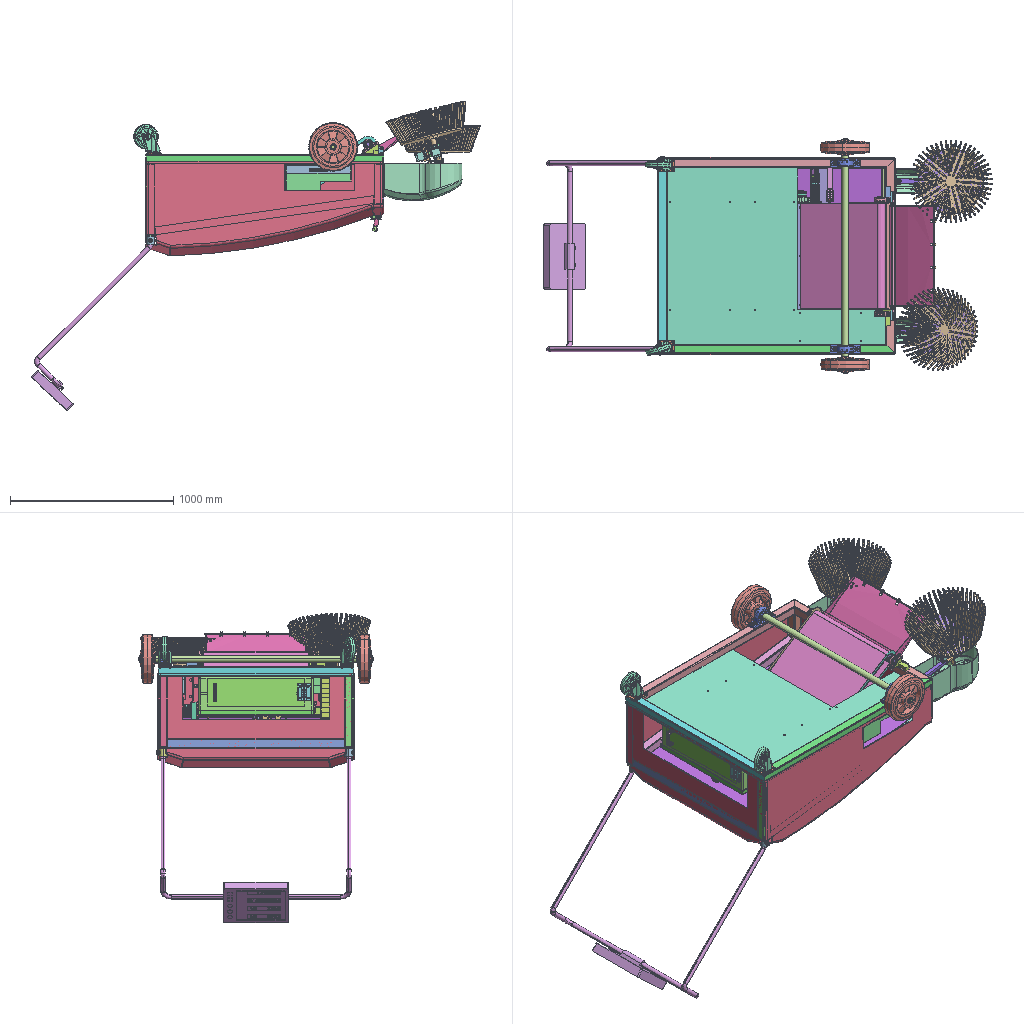Assembly | SolidWorks | 107 different items | 175 placed | box 2749 x 1446 x 1897 mm
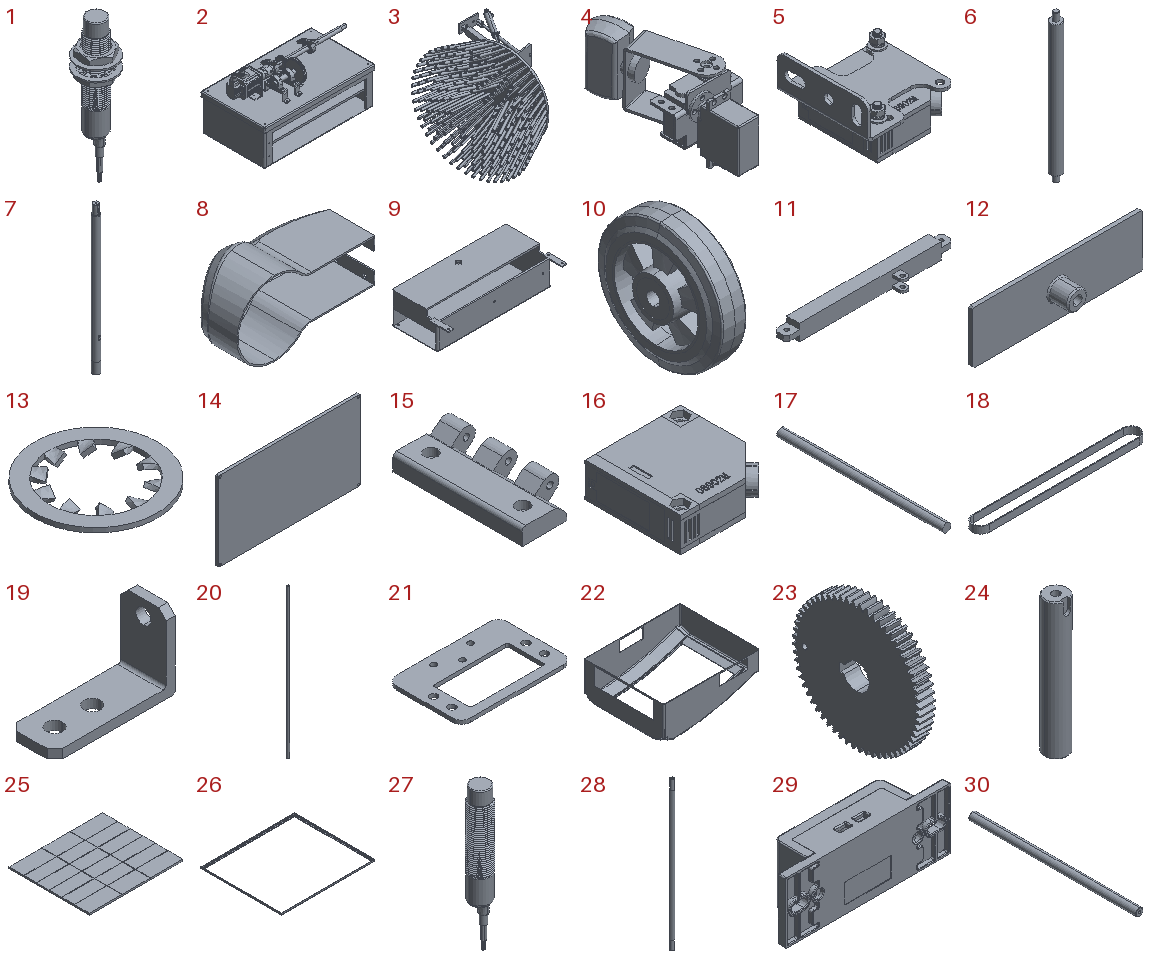Parts list (item | name | quantity | parent item | size | volume | features):
1 | (subassembly) | x1 | - | 21.5 x 21.5 x 81 mm | 7129 mm3 | features CompositeCurve 7
2 | (subassembly) | x1 | - | 752 x 410 x 396 mm | 13592742 mm3 | features CompositeCurve 2
3 | (subassembly) | x1 | - | 492.003 x 639.962 x 507.373 mm | 6091751 mm3 | -
4 | (subassembly) | x1 | - | 62.179 x 144.352 x 61.763 mm | 114357 mm3 | features MirrorCompFeat 1
5 | (subassembly) | x1 | - | 60 x 58 x 40 mm | 49039 mm3 | features CompositeCurve 4
6 | - | x1 | - | 55 x 55 x 730 mm | 1583008 mm3 | features Chamfer 1, Extrusion 1, ICE 1, MirrorPattern 1
7 | - | x1 | - | 25 x 25 x 522 mm | 247598 mm3 | features ICE 4, Chamfer 1, Extrusion 1, Fillet 1, HoleWzd 1
8 | - | x2 | - | 480 x 231.625 x 260 mm | 1531770 mm3 | features Fillet 2, ICE 2, Chamfer 1, Extrusion 1, Shell 1
9 | - | x1 | - | 730 x 359.087 x 200 mm | 6377520 mm3 | features ICE 5, HoleWzd 3, Extrusion 1, Fillet 1, Shell 1
10 | - | x2 | - | 90 x 300 x 300 mm | 3470694 mm3 | features BaseBody 1, Scale 1
11 | - | x2 | - | 260 x 36.5 x 25 mm | 116892 mm3 | features ICE 3, Chamfer 1, Extrusion 1, LPattern 1, MirrorPattern 1
12 | - | x1 | - | 130 x 18 x 40 mm | 17593 mm3 | features Chamfer 1, Extrusion 1, HoleWzd 1, ICE 1
13 | - | x2 | in 1 | 21.5 x 21.5 x 1.797 mm | 153.883 mm3 | features CirPattern 1, Extrusion 1, Helix 1, Sweep 1
14 | - | x1 | - | 680 x 47 x 380 mm | 3131077 mm3 | features ICE 5, Chamfer 1, Extrusion 1
15 | - | x2 | - | 47.1 x 102 x 20.1 mm | 51608 mm3 | features MBimport 1
16 | - | x1 | in 5 | 50 x 50 x 18 mm | 41624 mm3 | features ICE 29, LPattern 4, CirPattern 2, Fillet 2, Chamfer 1, Extrusion 1, MirrorPattern 1
17 | - | x1 | - | 5 x 99 x 5 mm | 1944 mm3 | features MBimport 1
18 | - | x1 | - | 667 x 67 x 27 mm | 113486 mm3 | features Extrusion 1
19 | - | x2 | - | 80 x 30 x 50 mm | 20408 mm3 | features Chamfer 1, Extrusion 1, Fillet 1, ICE 1
20 | - | x1 | - | 10 x 10 x 700 mm | 54949 mm3 | features Chamfer 1, Extrusion 1
21 | - | x1 | - | 60 x 40 x 2 mm | 2957 mm3 | features ICE 3, Extrusion 1
22 | - | x1 | - | 1460 x 1210 x 578.799 mm | 14635130 mm3 | features ICE 7, Chamfer 3, Fillet 2, MoveFace 2, Shell 1
23 | - | x1 | - | 15 x 123.892 x 123.892 mm | 159845 mm3 | features HoleWzd 1, MBimport 1
24 | - | x1 | - | 25 x 25 x 150 mm | 71725 mm3 | features Chamfer 1, Extrusion 1, Fillet 1, HoleWzd 1, ICE 1
25 | - | x1 | - | 1340 x 1150 x 55 mm | 38292286 mm3 | features ICE 3, Extrusion 1, LPattern 1, Sweep 1
26 | - | x1 | - | 1348 x 1158 x 25 mm | 890268 mm3 | features WeldMemberFeat 1, WeldmentFeature 1
27 | - | x1 | in 1 | 11.9 x 11.9 x 81 mm | 5802 mm3 | features Fillet 4, ICE 4, Revolution 4, Helix 1, SweepCut 1
28 | - | x1 | - | 40 x 40 x 1420 mm | 1677021 mm3 | features HoleWzd 2, Chamfer 1, Extrusion 1, ICE 1
29 | - | x1 | - | 40.625 x 10.25 x 15 mm | 2277 mm3 | features BaseBody 3, CombineBodies 1, MoveFace 1, Scale 1
30 | - | x4 | - | 10 x 220 x 10 mm | 17093 mm3 | features HoleWzd 2, Chamfer 1, Extrusion 1
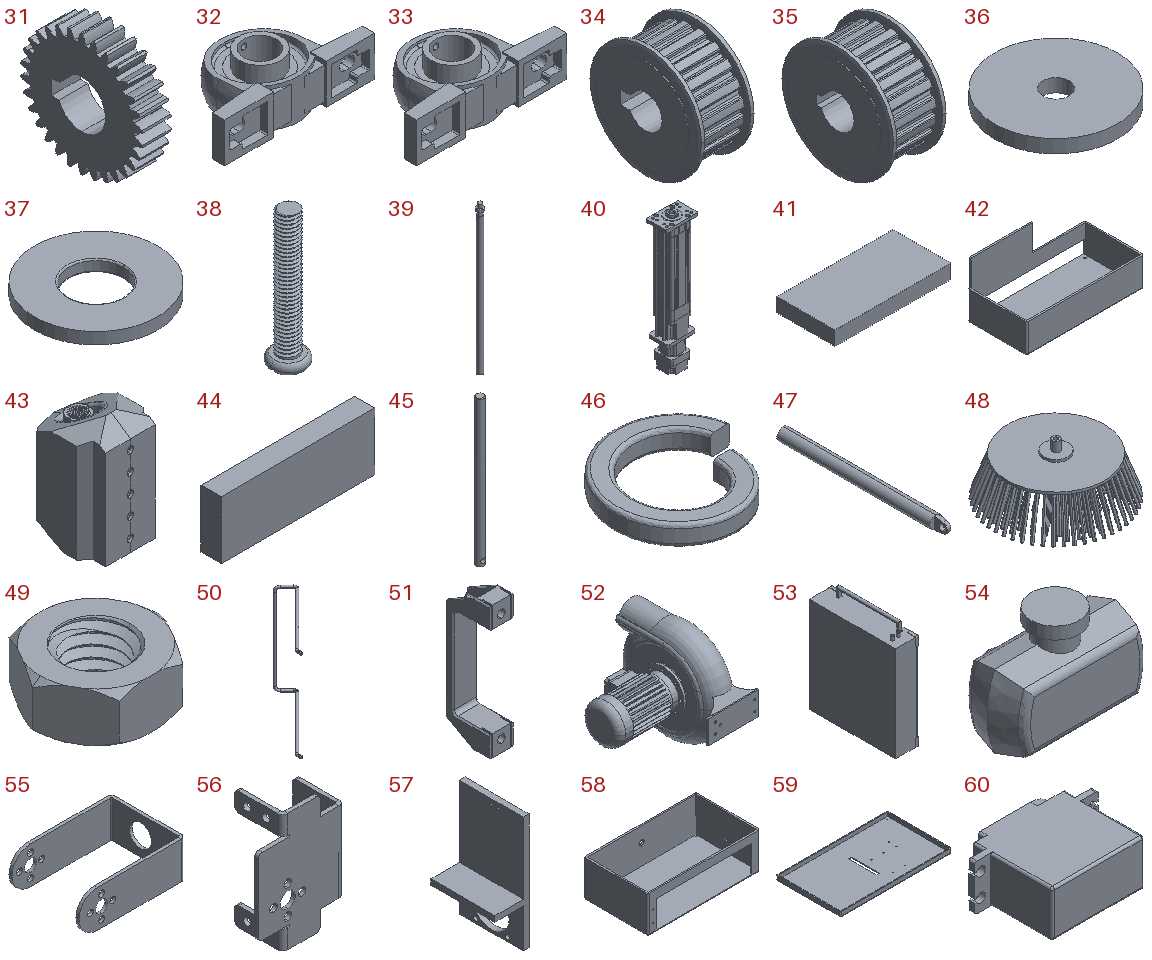31 | - | x1 | - | 15 x 63.764 x 64 mm | 33715 mm3 | features MBimport 1
32 | - | x2 | - | 186 x 100.8 x 54.842 mm | 267001 mm3 | features Revolution 5, Boss 3, Cut 3, RevCut 2, CirPattern 1, Extrusion 1, SweepCut 1
33 | - | x8 | - | 116.25 x 63 x 34.276 mm | 65186 mm3 | features Revolution 5, Boss 3, Cut 3, RevCut 2, CirPattern 1, Extrusion 1, Scale 1, SweepCut 1
34 | - | x1 | - | 32 x 67 x 67 mm | 76462 mm3 | features ICE 1, MBimport 1
35 | - | x2 | - | 32 x 67 x 67 mm | 77303 mm3 | features ICE 1, MBimport 1
36 | - | x2 | - | 28 x 28 x 3 mm | 1762 mm3 | features Extrusion 1
37 | - | x2 | in 5 | 9.05 x 9.05 x 0.85 mm | 43.941 mm3 | features Extrusion 1, Fillet 1, ICE 1
38 | - | x2 | in 5 | 6.8 x 6.8 x 27.2 mm | 311.216 mm3 | features ICE 4, Chamfer 1, Extrusion 1, Fillet 1, Helix 1, RevCut 1, Revolution 1, SweepCut 1
39 | - | x1 | - | 12 x 13.856 x 280 mm | 21775 mm3 | features MBimport 1, MoveFace 1, Scale 1
40 | - | x1 | - | 66 x 42 x 279.6 mm | 278895 mm3 | features MBimport 1, MoveFace 1
41 | - | x1 | - | 390 x 195 x 47.5 mm | 741654 mm3 | features Extrusion 1, Shell 1
42 | - | x1 | - | 400 x 200 x 190 mm | 953105 mm3 | features ICE 3, Fillet 2, Extrusion 1, Shell 1
43 | - | x1 | - | 45.232 x 51.14 x 74.295 mm | 38659 mm3 | features BaseBody 6
44 | - | x1 | - | 690 x 90 x 260 mm | 2021904 mm3 | features Extrusion 1, Shell 1
45 | - | x2 | - | 8 x 8 x 150 mm | 7385 mm3 | features Chamfer 1, Extrusion 1, ICE 1
46 | - | x2 | in 5 | 6.6 x 6.6 x 2.189 mm | 20.119 mm3 | features Helix 1, Sweep 1
47 | - | x2 | - | 12 x 163 x 12 mm | 9872 mm3 | features ICE 2, Extrusion 1, Shell 1
48 | - | x2 | - | - | - | features CirPattern 7, ICE 3, CombineBodies 1, Extrusion 1, Fillet 1, LPattern 1, OffsetRefSurface 1, ReplaceFace 1, Sweep 1
49 | - | x2 | in 5 | 7.91 x 6.85 x 3.05 mm | 87.239 mm3 | features Chamfer 1, Extrusion 1, Helix 1, ICE 1, RevCut 1, SweepCut 1
50 | - | x1 | - | 724.68 x 923.528 x 1170 mm | 1404787 mm3 | features 3DProfileFeature 3, Cut 1, Shell 1, Sweep 1
51 | - | x3 | - | 20 x 36 x 110 mm | 17645 mm3 | features MBimport 1
52 | - | x1 | - | - | - | features DeleteBody 6, MoveCopyBody 4, MBimport 1, Scale 1
53 | - | x1 | - | 36 x 137.7 x 182.4 mm | 710177 mm3 | features ICE 1, MBimport 1, Scale 1
54 | - | x1 | in 4 | - | - | features ICE 4, Fillet 3, Extrusion 1, RevolvRefSurf 1
55 | - | x1 | in 4 | 71.712 x 49.895 x 25 mm | 8226 mm3 | features ICE 3, FlatPattern 1, SM3dBend 1, SMBaseFlange 1, SheetMetal 1
56 | - | x1 | in 4 | 45 x 25 x 62 mm | 6846 mm3 | features ICE 5, Fillet 3, EdgeFlange 2, SMBaseFlange 2, FlatPattern 1, MirrorPattern 1, SheetMetal 1
57 | - | x2 | - | 48 x 90 x 163 mm | 129456 mm3 | features ICE 3, Cut 2, Extrusion 1, HoleWzd 1
58 | - | x1 | - | 700 x 400 x 230 mm | 6454208 mm3 | features Cut 4, HoleWzd 3, Extrusion 1, Fillet 1, Shell 1
59 | - | x1 | - | 710 x 410 x 30 mm | 1701440 mm3 | features Cut 1, Extrusion 1, Fillet 1, HoleWzd 1, ICE 1, Shell 1
60 | - | x2 | in 4 | 54 x 43 x 20 mm | 30390 mm3 | features ICE 5, 3DProfileFeature 1, Extrusion 1, Fillet 1, HoleWzd 1
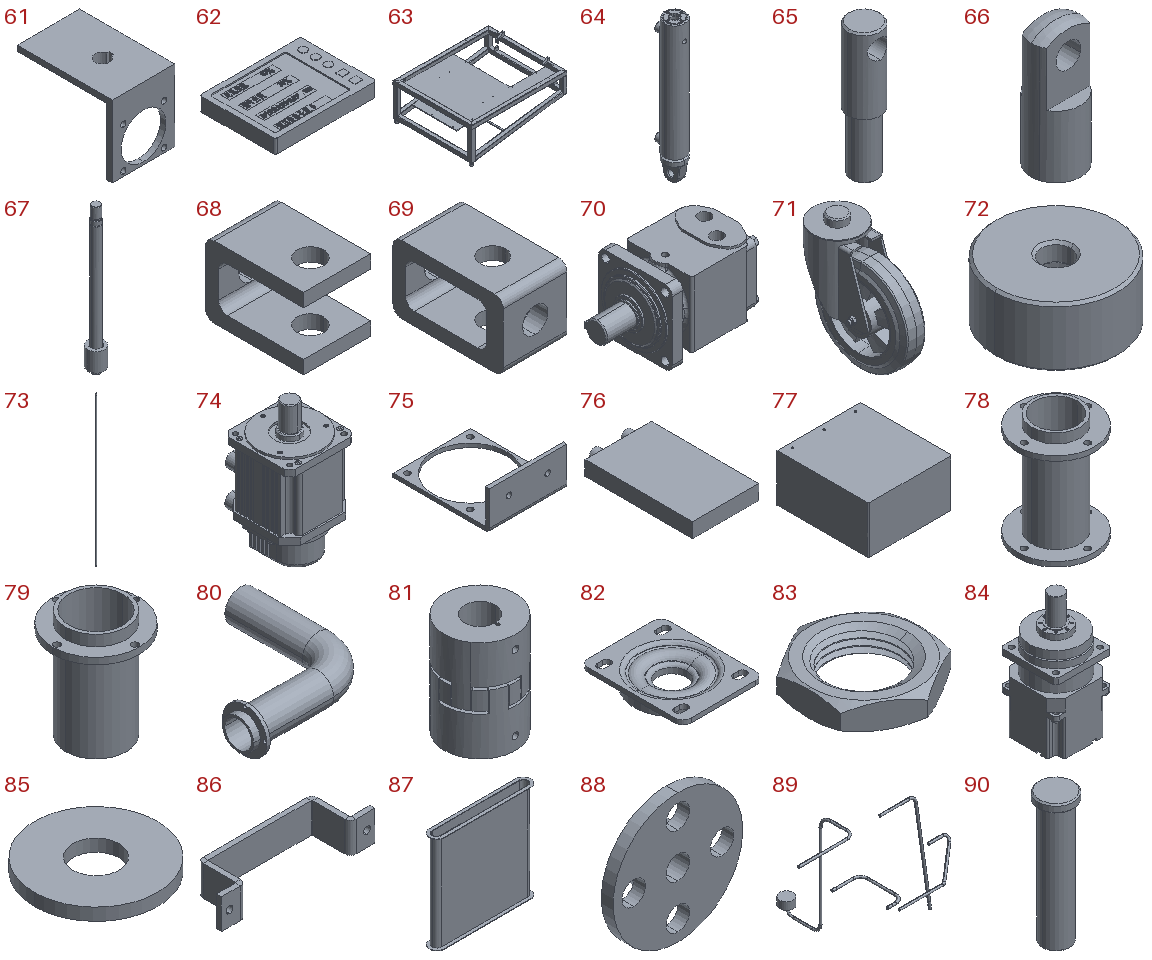61 | - | x2 | - | 70 x 106 x 80 mm | 69922 mm3 | features ICE 3, Cut 1, Extrusion 1
62 | - | x1 | - | 400 x 300 x 104.5 mm | 6453312 mm3 | features ICE 7, Extrusion 1, Fillet 1, HoleWzd 1
63 | - | x1 | - | 1460 x 1200 x 621.009 mm | 23985037 mm3 | features ICE 14, MoveCopyBody 6, WeldMemberFeat 4, Fillet 3, HoleWzd 3, BossThin 2, Cut 2, EndCap 2, MirrorSolid 2, WeldCornerFeat 2, WeldmentFeature 1
64 | - | x2 | - | 22 x 28 x 150.8 mm | 29606 mm3 | features BaseBody 4, CombineBodies 1, Scale 1
65 | - | x1 | - | 10 x 10 x 41 mm | 2435 mm3 | features ICE 2, Chamfer 1, Extrusion 1
66 | - | x2 | - | 12 x 12 x 30 mm | 1906 mm3 | features MBimport 1, MoveFace 1, Scale 1
67 | - | x2 | - | 15.92 x 15.92 x 140.8 mm | 10674 mm3 | features BaseBody 2, CombineBodies 1, Scale 1
68 | - | x1 | - | 15 x 22 x 16 mm | 2176 mm3 | features ICE 2, Extrusion 1, Fillet 1
69 | - | x1 | - | 15 x 26 x 16 mm | 3022 mm3 | features ICE 3, Fillet 2, Extrusion 1
70 | - | x4 | - | 102 x 56 x 56 mm | 177748 mm3 | features ICE 1, MBimport 1, Scale 1
71 | - | x2 | - | 77.25 x 166.125 x 185.063 mm | 534809 mm3 | features BaseBody 4, CombineBodies 2, ICE 2, Chamfer 1, MoveCopyBody 1, MoveFace 1, Scale 1
72 | - | x4 | - | 25 x 25 x 12 mm | 4138 mm3 | features Chamfer 1, Cut 1, Extrusion 1
73 | - | x1 | - | 5 x 5 x 632 mm | 12318 mm3 | features Chamfer 1, Extrusion 1, ICE 1, MirrorPattern 1
74 | - | x1 | - | 100 x 136 x 194 mm | 1174921 mm3 | features ICE 1, MBimport 1
75 | - | x1 | - | 100 x 125 x 50 mm | 47710 mm3 | features Cut 1, EdgeFlange 1, FlatPattern 1, ICE 1, SMBaseFlange 1, SheetMetal 1
76 | - | x8 | - | 135 x 235 x 30 mm | 903464 mm3 | features Extrusion 1, ICE 1
77 | - | x1 | - | 252 x 276 x 143 mm | 499174 mm3 | features SMBaseFlange 3, SheetMetal 3, CombineBodies 1, Cut 1, Fillet 1, FlatPattern 1, HoleWzd 1
78 | - | x1 | - | 80 x 80 x 120 mm | 82655 mm3 | features Extrusion 1, ICE 1, MirrorPattern 1
79 | - | x1 | - | 40 x 40 x 50 mm | 8082 mm3 | features Extrusion 1, ICE 1
80 | - | x1 | - | 116 x 120 x 40 mm | 32734 mm3 | features ICE 1, Shell 1, Sweep 1
81 | - | x1 | - | 55 x 55 x 78 mm | 139645 mm3 | features ICE 1, MBimport 1
82 | - | x2 | - | 82.5 x 105 x 14.438 mm | 61756 mm3 | features BaseBody 4, CombineBodies 2, ICE 2, MoveCopyBody 1, MoveFace 1, Scale 1
83 | - | x2 | in 1 | 16.5 x 19.053 x 4 mm | 509.412 mm3 | features Helix 1, ICE 1, RevCut 1, Revolution 1, SweepCut 1
84 | - | x1 | - | 30 x 37.375 x 65.875 mm | 38357 mm3 | features BaseBody 3, CombineBodies 1, Scale 1
85 | - | x2 | - | 40 x 40 x 4 mm | 4320 mm3 | features Extrusion 1
86 | - | x2 | - | 156.25 x 44.25 x 30.75 mm | 34854 mm3 | features FlatPattern 1, ICE 1, SMBaseFlange 1, SheetMetal 1
87 | - | x1 | - | 680 x 100 x 650 mm | 2347902 mm3 | features Extrusion 1, ICE 1, MirrorSolid 1
88 | - | x2 | in 4 | 22 x 6 x 22 mm | 838.805 mm3 | features ICE 2, Extrusion 1
89 | - | x1 | - | 155.715 x 218.5 x 171.95 mm | 7637 mm3 | features 3DProfileFeature 5, Sweep 4, ICE 1
90 | - | x1 | - | 13 x 13 x 48 mm | 3919 mm3 | features Chamfer 1, Extrusion 1, ICE 1
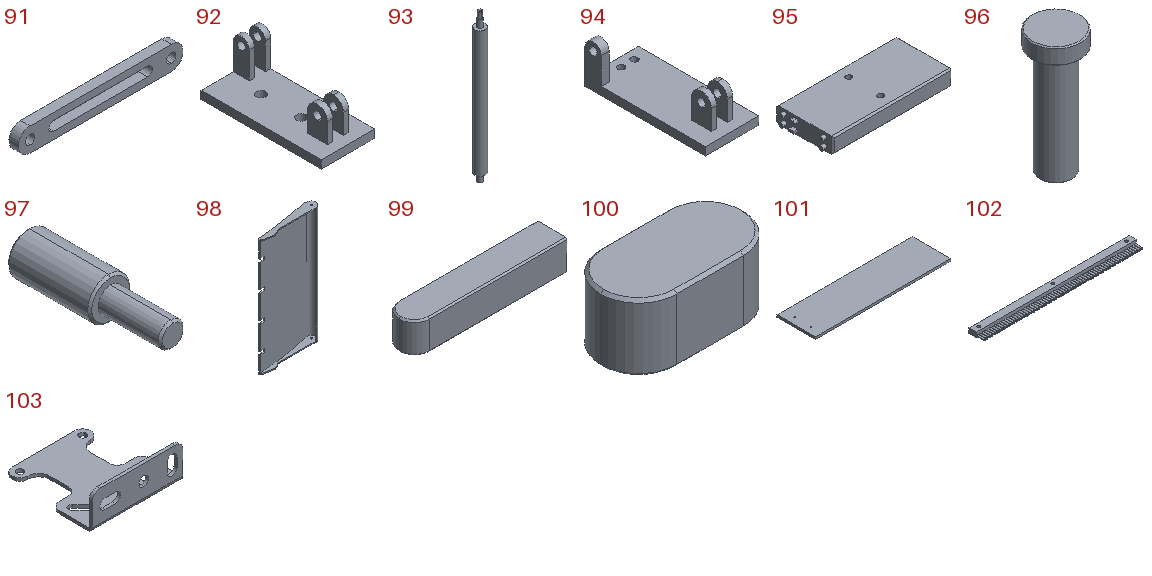91 | - | x1 | - | 175 x 10 x 25 mm | 30053 mm3 | features Extrusion 1, ICE 1
92 | - | x2 | - | 40 x 90 x 32 mm | 25565 mm3 | features ICE 3, Extrusion 1, LPattern 1, MirrorPattern 1
93 | - | x1 | - | 55 x 55 x 762 mm | 1592560 mm3 | features ICE 3, Chamfer 2, Extrusion 1, HoleWzd 1, MirrorPattern 1
94 | - | x2 | - | 40 x 90 x 32 mm | 25255 mm3 | features ICE 3, Extrusion 1, MirrorPattern 1
95 | - | x1 | - | 155 x 70 x 20 mm | 207430 mm3 | features ICE 2, Chamfer 1, Extrusion 1
96 | - | x12 | - | 9 x 9 x 23 mm | 754.856 mm3 | features Chamfer 1, Extrusion 1, ICE 1
97 | - | x1 | - | 10 x 35 x 10 mm | 1985 mm3 | features Chamfer 1, Extrusion 1, ICE 1
98 | - | x1 | - | 325.159 x 69.885 x 620 mm | 1237275 mm3 | features Fillet 3, ICE 3, Extrusion 1, MirrorPattern 1, Shell 1
99 | - | x2 | - | 30 x 6 x 6 mm | 1051 mm3 | features Chamfer 1, Extrusion 1, Fillet 1
100 | - | x2 | - | 15 x 8 x 7 mm | 740.393 mm3 | features Chamfer 1, Extrusion 1, Fillet 1
101 | - | x1 | - | 600 x 170 x 10 mm | 1019607 mm3 | features Extrusion 1, HoleWzd 1
102 | - | x1 | - | 650 x 60 x 20 mm | 429985 mm3 | features ICE 3, Fillet 2, Extrusion 1, LPattern 1, Sweep 1
103 | - | x1 | in 5 | 58 x 60 x 22 mm | 6510 mm3 | features ICE 3, MirrorPattern 2, SketchHole 2, EdgeFlange 1, Fillet 1, FlatPattern 1, SMBaseFlange 1, SheetMetal 1
104 | deep groove ball bearings gb | x1 | - | - | - | -
105 | hex nuts, style 1-grades ab gb | x1 | - | - | - | -
106 | hexagon head bolts-full thread gb | x1 | - | - | - | -
107 | hexagon socket head cap screws gb | x1 | - | - | - | -
Mates (type | each side: item.copy, entity, surface, feature):
In the top assembly
Coincident | 63.1 plane | assembly plane | 6 times
Width | 25.1 face plane Boss-Extrude1 | 25.1 face plane Boss-Extrude1 | 63.1 face plane Square tube - configured 80 X 80 X 5(4) | 63.1 face plane Body-Move/Copy5
Width | 9.1 face plane Boss-Extrude1 | 9.1 face plane Boss-Extrude1 | 63.1 face plane Square tube - configured 80 X 80 X 5(1) | 63.1 face plane Square tube - configured 80 X 80 X 5(1)
Concentric | 10.1 face cylinder RE.G2-200-RSL.step-1/RE-G2-L.step-1-solid1 | 10.2 face cylinder RE.G2-200-RSL.step-1/RE-G2-L.step-1-solid1
DistanceDim | 10.1 face plane RE.G2-200-RSL.step-1/RE-G2-L.step-1-solid1 | 63.1 face plane Square tube - configured 80 X 80 X 5(1)
DistanceDim | 10.2 face plane RE.G2-200-RSL.step-1/RE-G2-L.step-1-solid1 | 63.1 face plane Square tube - configured 80 X 80 X 5(1)
Concentric | 10.1 face cylinder RE.G2-200-RSL.step-1/RE-G2-L.step-1-solid1 | 28.1 face cylinder Boss-Extrude3
Width | 28.1 face plane Boss-Extrude1 | 28.1 face plane Boss-Extrude1 | 10.2 face plane RE.G2-200-RSL.step-1/RE-G2-L.step-1-solid1 | 10.1 face plane RE.G2-200-RSL.step-1/RE-G2-L.step-1-solid1
Concentric | 32.1 face cylinder Boss-Revolve5 | 28.1 face cylinder Boss-Extrude3
Concentric | 28.1 face cylinder Boss-Extrude3 | 32.2 face cylinder Boss-Revolve5
Coincident | 32.1 face plane Boss-Extrude1 | 32.2 face plane Boss-Extrude1
Coincident | 63.1 face plane Square tube - configured 80 X 80 X 5(1) | 32.1 face plane Boss-Extrude1
Width | 32.1 face plane Boss-Extrude1 | 32.1 face plane Boss-Extrude1 | 63.1 face plane Square tube - configured 80 X 80 X 5(1) | 63.1 face plane Square tube - configured 80 X 80 X 5(1)
Width | 32.2 face plane Boss-Extrude1 | 32.2 face plane Boss-Extrude1 | 63.1 face plane Square tube - configured 80 X 80 X 5(1) | 63.1 face plane Square tube - configured 80 X 80 X 5(1)
Width | 87.1 face plane Boss-Extrude1 | 87.1 face plane Boss-Extrude1 | 63.1 face plane Square tube - configured 80 X 80 X 5(4) | 63.1 face plane Body-Move/Copy5
Concentric | 87.1 face cylinder Boss-Extrude1 | 6.1 face cylinder Boss-Extrude1
Coincident | 87.1 face plane Boss-Extrude1 | 6.1 face plane Boss-Extrude1
Concentric | 87.1 face cylinder Boss-Extrude1 | 93.1 face cylinder Boss-Extrude1
Coincident | 87.1 face plane Boss-Extrude1 | 93.1 face plane Boss-Extrude1
Concentric | 6.1 face cylinder Boss-Extrude2 | 33.1 face cylinder Boss-Revolve5
Concentric | 6.1 face cylinder Mirror1 | 33.2 face cylinder Boss-Revolve5
Coincident | 33.2 face plane Boss-Extrude1 | 33.1 face plane Boss-Extrude1
Coincident | 6.1 face plane Boss-Extrude2 | 33.1 face plane Boss-Revolve5
Coincident | 6.1 face plane Mirror1 | 33.2 face plane Boss-Revolve5
Concentric | 93.1 face cylinder Boss-Extrude2 | 33.3 face cylinder Boss-Revolve5
Concentric | 93.1 face cylinder Mirror1 | 33.4 face cylinder Boss-Revolve5
Coincident | 33.3 face plane Boss-Extrude1 | 33.4 face plane Boss-Extrude1
Coincident | 93.1 face plane Boss-Extrude2 | 33.3 face plane Boss-Revolve5
Coincident | 93.1 face plane Mirror1 | 33.4 face plane Boss-Revolve5
Parallel | 63.1 face plane Square tube - configured 80 X 80 X 5(1) | 33.3 face plane Boss-Extrude1
Coincident | 76.1 face plane Boss-Extrude1 | 77.1 face plane Base-Flange1 | 2 times
Coincident | 76.1 face plane Boss-Extrude1 | 77.1 face plane Base-Flange3
Concentric | 63.1 face cylinder Boss-Extrude1 | 50.1 face cylinder Sweep1 | 2 times
Coincident | 63.1 face plane Square tube - configured 80 X 80 X 5(3) | 50.1 face plane Sweep1
Coincident | 71.1 face plane Cut-Extrude1 | 82.1 face plane Caster with Brake.STEP-1/RE.G2-200-SSF-H.step.STEP-1/RE-G2-SSF-H-ZL.step.STEP-1-solid1
Concentric | 71.1 face cylinder Caster with Brake.STEP-1/RE.G2-200-SSF-H.step.STEP-1/RE-G2-SSF-H-ZL.step.STEP-1-solid1 | 82.1 face cylinder Caster with Brake.STEP-1/RE.G2-200-SSF-H.step.STEP-1/RE-G2-SSF-H-ZL.step.STEP-1-solid1
Coincident | 63.1 face plane Square tube - configured 80 X 80 X 5(1) | 82.1 face plane Caster with Brake.STEP-1/RE.G2-200-SSF-H.step.STEP-1/RE-G2-SSF-H-ZL.step.STEP-1-solid1 | 3 times
Coincident | 71.2 face plane Cut-Extrude1 | 82.2 face plane Caster with Brake.STEP-1/RE.G2-200-SSF-H.step.STEP-1/RE-G2-SSF-H-ZL.step.STEP-1-solid1
Concentric | 71.2 face cylinder Caster with Brake.STEP-1/RE.G2-200-SSF-H.step.STEP-1/RE-G2-SSF-H-ZL.step.STEP-1-solid1 | 82.2 face cylinder Caster with Brake.STEP-1/RE.G2-200-SSF-H.step.STEP-1/RE-G2-SSF-H-ZL.step.STEP-1-solid1
Coincident | 63.1 face plane Square tube - configured 80 X 80 X 5(1) | 82.2 face plane Caster with Brake.STEP-1/RE.G2-200-SSF-H.step.STEP-1/RE-G2-SSF-H-ZL.step.STEP-1-solid1 | 3 times
Width | 102.1 face plane Boss-Extrude1 | 102.1 face plane Boss-Extrude1 | 63.1 face plane Square tube - configured 80 X 80 X 5(4) | 63.1 face plane Body-Move/Copy5
Coincident | 9.1 face plane Boss-Extrude1 | 58.1 face plane Boss-Extrude1 | 2 times
Width | 98.1 face plane Boss-Extrude2 | 98.1 face plane Boss-Extrude2 | 63.1 face plane Square tube - configured 80 X 80 X 5(2) | 63.1 face plane Body-Move/Copy1
Concentric | 98.1 face cylinder Cut-Extrude1 | 73.1 face cylinder Boss-Extrude1
Coincident | 98.1 face plane Boss-Extrude2 | 73.1 edge
Concentric | 73.1 face cylinder Boss-Extrude1 | 72.1 face cylinder Boss-Extrude1
Concentric | 73.1 face cylinder Boss-Extrude1 | 72.2 face cylinder Boss-Extrude1
Concentric | 73.1 face cylinder Boss-Extrude1 | 72.3 face cylinder Boss-Extrude1
Concentric | 73.1 face cylinder Boss-Extrude1 | 72.4 face cylinder Boss-Extrude1
DistanceDim | 72.2 face plane Boss-Extrude1 | 72.1 face plane Boss-Extrude1
DistanceDim | 72.4 face plane Boss-Extrude1 | 72.3 face plane Boss-Extrude1
DistanceDim | 72.3 face plane Boss-Extrude1 | 72.2 face plane Boss-Extrude1
Width | 72.4 face plane Boss-Extrude1 | 72.1 face plane Boss-Extrude1 | 98.1 face plane Boss-Extrude2 | 98.1 face plane Boss-Extrude2
Coincident | 58.1 face plane Shell1 | 14.1 face plane Boss-Extrude1 | 2 times
Coincident | 28.1 face plane Boss-Extrude1 | 85.1 face plane Boss-Extrude1
Concentric | 28.1 face cylinder M14 Tapped Hole2 | 85.1 face cylinder Boss-Extrude1
Coincident | 28.1 face plane Boss-Extrude1 | 85.2 face plane Boss-Extrude1
Concentric | 28.1 face cylinder M14 Tapped Hole1 | 85.2 face cylinder Boss-Extrude1
Coincident | 25.1 face plane Boss-Extrude1 | 26.1 face plane Angle iron - configured 25 X 25 X 4(1) | 3 times
Coincident | 63.1 face plane Body-Move/Copy5 | 26.1 face plane Angle iron - configured 25 X 25 X 4(1)
Concentric | 14.1 face cylinder Cut-Extrude1 | 91.1 face cylinder Boss-Extrude1
Coincident | 14.1 face plane Cut-Extrude2 | 91.1 face plane Boss-Extrude1
Coincident | 58.1 face plane Boss-Extrude1 | 59.1 face plane Shell1 | 3 times
Coincident | 63.1 face plane Square tube - configured 80 X 80 X 5(1) | 58.1 face plane Boss-Extrude1
Coincident | 63.1 face plane Body-Move/Copy1 | 58.1 face plane Boss-Extrude1
Coincident | 63.1 face plane Square tube - configured 80 X 80 X 5(1) | 77.1 face plane Base-Flange1
Coincident | 63.1 face plane Square tube - configured 80 X 80 X 5(2) | 77.1 face plane Base-Flange1
Concentric | 93.1 face cylinder Boss-Extrude3 | 35.1 face cylinder TAAL-20-100-H20.step
Coincident | 93.1 face plane Boss-Extrude3 | 35.1 face plane TAAL-20-100-H20.step
Coincident | 93.1 face plane Cut-Extrude1 | 35.1 face plane Cut-Extrude1
Concentric | 93.1 face cylinder Cut-Extrude1 | 99.1 face cylinder Fillet1
Coincident | 93.1 face plane Cut-Extrude1 | 99.1 face plane Boss-Extrude1 | 2 times
Coincident | 93.1 face plane Boss-Extrude3 | 36.1 face plane Boss-Extrude1
Concentric | 93.1 face cylinder M5 Tapped Hole1 | 36.1 face cylinder Boss-Extrude1
DistanceDim | 28.1 face cylinder Boss-Extrude3 | 63.1 face plane Square tube - configured 80 X 80 X 5(1)
Concentric | 50.1 face cylinder Sweep1 | 62.1 face cylinder Boss-Extrude7
Width | 62.1 face plane Boss-Extrude1 | 62.1 face plane Boss-Extrude1 | 63.1 face plane Square tube - configured 80 X 80 X 5(1) | 63.1 face plane Square tube - configured 80 X 80 X 5(1)
Concentric | 35.2 face cylinder TAAL-20-100-H20.step | 7.1 face cylinder Boss-Extrude2
Coincident | 35.2 face plane TAAL-20-100-H20.step | 7.1 face plane Boss-Extrude2
Concentric | 74.1 face cylinder SGMSH-10AA A.STEP | 7.1 face cylinder Boss-Extrude1
Coincident | 35.1 face plane TAAL-20-100-H20.step | 35.2 face plane TAAL-20-100-H20.step
Concentric | 7.1 face cylinder Boss-Extrude1 | 31.1 face cylinder Small Gear.STEP
Coincident | 91.1 face plane Boss-Extrude1 | 97.1 face plane Boss-Extrude1
Concentric | 23.1 face cylinder M6 Tapped Hole1 | 97.1 face cylinder Boss-Extrude2
Coincident | 91.1 face plane Boss-Extrude1 | 23.1 face plane Large Gear.STEP
Coincident | 23.1 face plane Large Gear.STEP | 31.1 face plane Small Gear.STEP
DistanceDim | 31.1 face cylinder Small Gear.STEP | 23.1 face cylinder Large Gear.STEP
DistanceDim | 23.1 face cylinder Large Gear.STEP | 58.1 face plane Boss-Extrude1
Parallel | 59.1 face plane Boss-Extrude1 | 74.1 face plane SGMSH-10AA A.STEP
DistanceDim | 23.1 face cylinder Large Gear.STEP | 63.1 face plane Square tube - configured 80 X 80 X 5(1)
DistanceDim | 31.1 face cylinder Small Gear.STEP | 63.1 face plane Square tube - configured 80 X 80 X 5(1)
Concentric | 7.1 face cylinder Boss-Extrude1 | 33.5 face cylinder Boss-Revolve5
Concentric | 7.1 face cylinder Boss-Extrude1 | 33.6 face cylinder Boss-Revolve5
Coincident | 33.5 face plane Boss-Extrude1 | 33.6 face plane Boss-Extrude1
Coincident | 63.1 face plane Square tube - configured 80 X 80 X 5(2) | 77.1 face plane Base-Flange2
Coincident | 7.1 face plane Boss-Extrude2 | 36.2 face plane Boss-Extrude1
Concentric | 7.1 edge | 36.2 face cylinder Boss-Extrude1
Coincident | 35.2 face plane Cut-Extrude1 | 7.1 face plane Cut-Extrude1
Coincident | 7.1 face plane Cut-Extrude1 | 99.2 face plane Boss-Extrude1 | 2 times
Coincident | 7.1 face plane Boss-Extrude2 | 99.2 face plane Boss-Extrude1
Parallel | 63.1 face plane Body-Move/Copy5 | 33.5 face plane Boss-Extrude1
GearDim | 31.1 face cylinder Small Gear.STEP | 23.1 face cylinder Large Gear.STEP
Coincident | 7.1 face plane Boss-Extrude1 | 33.6 face plane Boss-Revolve5
Concentric | 23.1 face cylinder Large Gear.STEP | 24.1 face cylinder Boss-Extrude1
Concentric | 24.1 face cylinder Boss-Extrude1 | 33.7 face cylinder Boss-Revolve5
Concentric | 24.1 face cylinder Boss-Extrude1 | 33.8 face cylinder Boss-Revolve5
Coincident | 24.1 face plane Boss-Extrude1 | 33.8 face plane Boss-Revolve5
Coincident | 33.7 face plane Boss-Extrude1 | 33.8 face plane Boss-Extrude1
Parallel | 59.1 face plane Boss-Extrude1 | 33.8 face plane Boss-Extrude1
Coincident | 33.7 face plane Boss-Extrude1 | 86.1 face plane Base-Flange1 | 3 times
Coincident | 33.8 face plane Boss-Extrude1 | 86.2 face plane Base-Flange1 | 3 times
Concentric | 74.1 face cylinder SGMSH-10AA A.STEP | 81.1 face cylinder Cut-Extrude1
Coincident | 7.1 face plane Boss-Extrude3 | 81.1 edge
Coincident | 74.1 face plane SGMSH-10AA A.STEP | 81.1 edge
Concentric | 14.1 face cylinder Cut-Extrude1 | 90.1 face cylinder Boss-Extrude1
Tangent | 14.1 face cylinder Boss-Extrude2 | 90.1 face plane Boss-Extrude2
Coincident | 23.1 face plane Large Gear.STEP | 24.1 face plane Boss-Extrude1
DistanceDim | 33.7 face plane Boss-Revolve5 | 23.1 face plane Large Gear.STEP
Coincident | 23.1 face plane Large Gear.STEP | 24.1 face plane Cut-Extrude1
Coincident | 23.1 face plane Large Gear.STEP | 100.1 face plane Boss-Extrude1 | 2 times
Concentric | 24.1 face cylinder Fillet1 | 100.1 face cylinder Fillet1
Coincident | 31.1 face plane Small Gear.STEP | 100.2 face plane Boss-Extrude1 | 2 times
Coincident | 31.1 face plane Small Gear.STEP | 100.2 edge
Coincident | 74.1 face plane SGMSH-10AA A.STEP | 75.1 face plane Base-Flange1 | 2 times
Coincident | 74.1 edge | 75.1 face plane Base-Flange1
Concentric | 7.1 face cylinder Boss-Extrude1 | 18.1 face cylinder Boss-Extrude1
Tangent | 35.2 face torus TAAL-20-100-H20.step | 18.1 face plane Boss-Extrude1
Concentric | 93.1 face cylinder Boss-Extrude2 | 18.1 face cylinder Boss-Extrude1
DistanceDim | 9.1 face plane Boss-Extrude1 | 33.3 face plane Boss-Extrude1
Coincident | 9.1 face plane Boss-Extrude1 | 33.3 face plane Boss-Extrude1
Coincident | 63.1 edge | 26.1 face plane Angle iron - configured 25 X 25 X 4(1)
Concentric | 9.1 face cylinder Cut-Extrude2 | 52.1 face cylinder _GFJ.stp
Parallel | 63.1 face plane Body-Move/Copy5 | 52.1 face plane _GFJ.stp
Concentric | 9.1 face cylinder Cut-Extrude2 | 79.1 face cylinder Boss-Extrude1
Coincident | 9.1 face plane Boss-Extrude1 | 79.1 edge
Concentric | 9.1 face cylinder M3 Tapped Hole1 | 79.1 face cylinder Boss-Extrude2
DistanceDim | 52.1 face plane _GFJ.stp | 79.1 face plane Boss-Extrude2
Concentric | 52.1 face cylinder _GFJ.stp | 80.1 face cylinder Sweep1
Parallel | 80.1 plane | assembly plane
DistanceDim | 80.1 face plane Sweep1 | 52.1 face plane _GFJ.stp
Concentric | 91.1 face cylinder Boss-Extrude1 | 97.1 edge
Concentric | 14.1 face cylinder Cut-Extrude3 | 30.1 face cylinder Boss-Extrude1
Concentric | 14.1 face cylinder Cut-Extrude3 | 30.2 face cylinder Boss-Extrude1
Concentric | 14.1 face cylinder Cut-Extrude3 | 30.3 face cylinder Boss-Extrude1
Concentric | 14.1 face cylinder Cut-Extrude3 | 30.4 face cylinder Boss-Extrude1
Coincident | 30.1 face plane Boss-Extrude1 | 30.4 face plane Boss-Extrude1
Coincident | 30.2 face plane Boss-Extrude1 | 30.3 face plane Boss-Extrude1
Coincident | 30.2 face plane Boss-Extrude1 | 30.4 face plane Boss-Extrude1
Coincident | 59.1 face plane Shell1 | 30.1 face plane Boss-Extrude1
Parallel | 87.1 face plane Boss-Extrude1 | 33.1 face plane Boss-Extrude1
Concentric | 98.1 face cylinder Cut-Extrude1 | 20.1 face cylinder Boss-Extrude1
Width | 20.1 face plane Boss-Extrude1 | 20.1 face plane Boss-Extrude1 | 98.1 face plane Boss-Extrude2 | 98.1 face plane Boss-Extrude2
Coincident | 63.1 face plane Square tube - configured 80 X 80 X 5(1) | 19.1 face plane Boss-Extrude1 | 2 times
Concentric | 20.1 face cylinder Boss-Extrude1 | 19.1 face cylinder Boss-Extrude2
DistanceDim | 19.1 face plane Boss-Extrude1 | 98.1 face plane Boss-Extrude2
Coincident | 63.1 face plane Square tube - configured 80 X 80 X 5(1) | 19.2 face plane Boss-Extrude1 | 2 times
DistanceDim | 19.2 face plane Boss-Extrude1 | 98.1 face plane Boss-Extrude2
Coincident | 9.1 face plane Boss-Extrude1 | 102.1 face plane Boss-Extrude2
DistanceDim | 102.1 face plane Boss-Extrude1 | 9.1 face plane Boss-Extrude1
PlanarAngleDim | assembly plane | 87.1 face plane Boss-Extrude1
Coincident | 58.1 face plane Cut-Extrude3 | 29.1 edge | 2 times
DistanceDim | 63.1 face plane Square tube - configured 80 X 80 X 5(3) | 43.1 face plane
PlanarAngleDim | assembly plane | 43.1 face plane
DistanceDim | 43.1 edge | 63.1 face plane Body-Move/Copy5
Coincident | 63.1 face plane Body-Move/Copy5 | 43.1 edge
Concentric | 48.1 face cylinder Cut-Extrude1 | 70.1 face cylinder BM-D160.STEP
Concentric | 48.2 face cylinder Cut-Extrude1 | 70.2 face cylinder BM-D160.STEP
Coincident | 48.1 face plane Boss-Extrude3 | 70.1 face plane BM-D160.STEP
Coincident | 48.2 face plane Boss-Extrude3 | 70.2 face plane BM-D160.STEP
Coincident | 57.1 face plane Boss-Extrude3 | 94.1 face plane Boss-Extrude1 | 2 times
Concentric | 11.1 face cylinder Cut-Extrude1 | 94.1 face cylinder Boss-Extrude3
Coincident | 11.1 face plane Mirror2 | 94.1 face plane Boss-Extrude3
Coincident | 57.2 face plane Boss-Extrude3 | 94.2 face plane Boss-Extrude1 | 2 times
Concentric | 11.2 face cylinder Cut-Extrude1 | 94.2 face cylinder Boss-Extrude3
Coincident | 11.2 face plane Mirror2 | 94.2 edge
Width | 94.2 face plane Boss-Extrude1 | 94.2 face plane Boss-Extrude1 | 57.2 face plane Boss-Extrude1 | 57.2 face plane Boss-Extrude1
Width | 94.1 face plane Boss-Extrude1 | 94.1 face plane Boss-Extrude1 | 57.1 face plane Boss-Extrude1 | 57.1 face plane Boss-Extrude1
Concentric | 11.1 face cylinder Cut-Extrude1 | 92.1 face cylinder Mirror1
Coincident | 11.1 edge | 92.1 face plane Boss-Extrude3
Concentric | 11.2 face cylinder Cut-Extrude1 | 92.2 face cylinder Mirror1
Coincident | 11.2 edge | 92.2 face plane Boss-Extrude3
Coincident | 63.1 face plane Square tube - configured 80 X 80 X 5(3) | 92.1 face plane Boss-Extrude1
Coincident | 63.1 face plane Square tube - configured 80 X 80 X 5(3) | 92.2 face plane Boss-Extrude1
Coincident | 92.1 face plane Boss-Extrude1 | 92.2 face plane Boss-Extrude1
DistanceDim | 63.1 face plane Square tube - configured 80 X 80 X 5(1) | 92.1 face plane Boss-Extrude1 | 2 times
DistanceDim | 92.2 face plane Boss-Extrude1 | 63.1 face plane Square tube - configured 80 X 80 X 5(1)
Concentric | 92.1 face cylinder Boss-Extrude2 | 45.1 face cylinder Cut-Extrude1
Tangent | 92.1 face plane LPattern1 | 45.1 face cylinder Boss-Extrude1
Concentric | 92.2 face cylinder LPattern1 | 45.2 face cylinder Cut-Extrude1
Tangent | 92.2 face plane Boss-Extrude2 | 45.2 face cylinder Boss-Extrude1
Concentric | 45.1 face cylinder Boss-Extrude1 | 47.1 face cylinder Boss-Extrude1
Concentric | 94.1 edge | 47.1 face cylinder Boss-Extrude2
Concentric | 45.2 face cylinder Boss-Extrude1 | 47.2 face cylinder Boss-Extrude1
Concentric | 94.2 face cylinder Boss-Extrude2 | 47.2 face cylinder Boss-Extrude2
Concentric | 64.1 face cylinder DG-J-40-E-E1-L-200.step-1/DG-J-40-101.step-1-solid1 | 67.1 face cylinder DG-J-40-E-E1-L-200.step-1/DG-J-40-103.step-1-solid1
Concentric | 64.2 face cylinder DG-J-40-E-E1-L-200.step-1/DG-J-40-101.step-1-solid1 | 67.2 face cylinder DG-J-40-E-E1-L-200.step-1/DG-J-40-103.step-1-solid1
Concentric | 67.1 face cylinder DG-J-40-E-E1-L-200.step-1/DG-J-40-102.step-1-solid1 | 66.1 face cylinder Joint.stp
Coincident | 67.1 face plane DG-J-40-E-E1-L-200.step-1/DG-J-40-102.step-1-solid1 | 66.1 face plane Joint.stp
Concentric | 67.2 face cylinder DG-J-40-E-E1-L-200.step-1/DG-J-40-102.step-1-solid1 | 66.2 face cylinder Joint.stp
Coincident | 67.2 edge | 66.2 face plane Joint.stp
Concentric | 11.1 face cylinder LPattern1 | 66.2 face cylinder Joint.stp
Width | 66.2 face plane Joint.stp | 66.2 face plane Joint.stp | 11.1 face plane LPattern1 | 11.1 face plane Boss-Extrude2
Concentric | 11.2 face cylinder LPattern1 | 66.1 face cylinder Joint.stp
Width | 66.1 face plane Joint.stp | 66.1 face plane Joint.stp | 11.2 face plane Boss-Extrude2 | 11.2 face plane LPattern1
Concentric | 11.1 face cylinder Boss-Extrude2 | 96.1 face cylinder Boss-Extrude1
Coincident | 11.1 face plane Boss-Extrude1 | 96.1 edge
Concentric | 92.1 face cylinder Mirror1 | 96.2 face cylinder Boss-Extrude1
Coincident | 92.1 face plane Mirror1 | 96.2 edge
Concentric | 94.1 face cylinder Boss-Extrude3 | 96.3 face cylinder Boss-Extrude1
Coincident | 94.1 face plane Boss-Extrude3 | 96.3 face plane Boss-Extrude2
Concentric | 47.1 face cylinder Boss-Extrude2 | 96.4 face cylinder Boss-Extrude1
Coincident | 47.1 face plane Boss-Extrude2 | 96.4 face plane Boss-Extrude2
Concentric | 11.2 face cylinder Boss-Extrude2 | 96.5 face cylinder Boss-Extrude1
Coincident | 11.2 face plane Boss-Extrude1 | 96.5 face plane Boss-Extrude2
Concentric | 94.2 face cylinder Boss-Extrude3 | 96.6 face cylinder Boss-Extrude1
Coincident | 94.2 face plane Boss-Extrude3 | 96.6 edge
Concentric | 47.2 face cylinder Boss-Extrude2 | 96.7 face cylinder Boss-Extrude1
Coincident | 47.2 face plane Boss-Extrude2 | 96.7 face plane Boss-Extrude2
Concentric | 92.2 face cylinder Mirror1 | 96.8 face cylinder Boss-Extrude1
Coincident | 92.2 face plane Mirror1 | 96.8 face plane Boss-Extrude2
Coincident | 58.1 face plane Boss-Extrude1 | 29.1 face plane Ultrasonic Sensor Kit_Ultrasonic Sensor Kit.step-1/ULTRASONIC-BOT.step-1-solid1
Coincident | 58.1 face plane Cut-Extrude4 | 101.1 face plane Boss-Extrude1
Coincident | 101.1 face plane Boss-Extrude1 | 51.1 face plane 90.STEP
DistanceDim | 51.1 face plane 90.STEP | 101.1 face plane Boss-Extrude1
Width | 51.1 face plane 90.STEP | 51.1 face plane 90.STEP | 101.1 face plane Boss-Extrude1 | 101.1 face plane Boss-Extrude1
Concentric | 15.1 face cylinder Hinge.stp | 15.2 face cylinder Hinge.stp
Coincident | 15.1 face plane Hinge.stp | 15.2 face plane Hinge.stp
Concentric | 17.1 face cylinder Hinge Pin.prt.stp | 15.2 face cylinder Hinge.stp
Coincident | 15.1 face plane Hinge.stp | 17.1 face plane Hinge Pin.prt.stp
Coincident | 58.1 face plane Boss-Extrude1 | 15.2 face plane Hinge.stp
Coincident | 101.1 face plane Boss-Extrude1 | 15.1 face plane Hinge.stp
Coincident | 58.1 face plane Cut-Extrude4 | 15.2 face plane Hinge.stp
DistanceDim | 101.1 face plane Boss-Extrude1 | 15.1 edge
Width | 15.1 face plane Hinge.stp | 15.1 face plane Hinge.stp | 101.1 face plane Boss-Extrude1 | 101.1 face plane Boss-Extrude1
Coincident | 9.1 face plane Shell1 | 44.1 face plane Boss-Extrude1 | 2 times
Coincident | 9.1 face plane Boss-Extrude1 | 44.1 face plane Boss-Extrude1
Coincident | 44.1 face plane Boss-Extrude1 | 51.2 face plane 90.STEP
Width | 51.2 face plane 90.STEP | 51.2 face plane 90.STEP | 9.1 face plane Boss-Extrude1 | 9.1 face plane Boss-Extrude1
Width | 51.2 face plane 90.STEP | 51.2 face plane 90.STEP | 44.1 face plane Boss-Extrude1 | 44.1 face plane Boss-Extrude1
Coincident | 63.1 face plane Square tube - configured 80 X 80 X 5(1) | 42.1 face plane Boss-Extrude1
DistanceDim | 42.1 face plane Boss-Extrude1 | 63.1 face plane Square tube - configured 80 X 80 X 5(2)
DistanceDim | 42.1 face plane Boss-Extrude1 | 87.1 edge
Coincident | 77.1 face plane Base-Flange1 | 53.1 face plane 120-450-400.step
Coincident | 63.1 face plane Square tube - configured 80 X 80 X 5(2) | 53.1 face plane 120-450-400.step
Tangent | 63.1 face plane Square tube - configured 80 X 80 X 5(2) | 53.1 face cylinder 120-450-400.step
Coincident | 77.1 face plane Base-Flange1 | 95.1 face plane Boss-Extrude1 | 2 times
Coincident | 77.1 face plane Base-Flange3 | 95.1 face plane Boss-Extrude1
Concentric | 39.1 face cylinder Foreign Object Removal Rod.stp | 40.1 face cylinder Foreign Object Removal Rod Body.stp
Coincident | 87.1 face plane Boss-Extrude1 | 40.1 face plane Foreign Object Removal Rod Body.stp
Coincident | 63.1 face plane Body-Move/Copy5 | 40.1 face plane Foreign Object Removal Rod Body.stp
DistanceDim | 40.1 edge | 63.1 face plane Square tube - configured 80 X 80 X 5(3)
Concentric | 39.1 face cylinder Foreign Object Removal Rod.stp | 12.1 face cylinder Boss-Extrude1
Coincident | 39.1 face plane Foreign Object Removal Rod.stp | 12.1 face plane Boss-Extrude1
Parallel | 40.1 edge | 12.1 face plane Boss-Extrude2
Concentric | 64.2 face cylinder DG-J-40-E-E1-L-200.step-1/DG-J-40-104.step-1-solid1 | 96.9 face cylinder Boss-Extrude1
Coincident | 64.2 face plane DG-J-40-E-E1-L-200.step-1/DG-J-40-104.step-1-solid1 | 96.9 face plane Boss-Extrude2
Concentric | 64.1 face cylinder DG-J-40-E-E1-L-200.step-1/DG-J-40-104.step-1-solid1 | 96.10 face cylinder Boss-Extrude1
Coincident | 64.1 face plane DG-J-40-E-E1-L-200.step-1/DG-J-40-104.step-1-solid1 | 96.10 face plane Boss-Extrude2
Concentric | 63.1 face cylinder Cut-Extrude6 | 96.9 face cylinder Boss-Extrude1
Concentric | 63.1 face cylinder Cut-Extrude6 | 96.10 face cylinder Boss-Extrude1
Coincident | 57.1 face plane Boss-Extrude1 | 70.3 face plane BM-D160.STEP
Coincident | 57.1 face plane Boss-Extrude3 | 70.3 face plane BM-D160.STEP
Width | 70.3 face plane BM-D160.STEP | 70.3 face plane BM-D160.STEP | 57.1 face plane Boss-Extrude1 | 57.1 face plane Boss-Extrude1
Coincident | 57.2 face plane Boss-Extrude1 | 70.4 face plane BM-D160.STEP
Coincident | 57.2 face plane Boss-Extrude3 | 70.4 face plane BM-D160.STEP
Width | 70.4 face plane BM-D160.STEP | 70.4 face plane BM-D160.STEP | 57.2 face plane Boss-Extrude1 | 57.2 face plane Boss-Extrude1
Concentric | 70.3 face cylinder BM-D160.STEP | 61.1 face cylinder Boss-Extrude1
Coincident | 57.1 face plane Boss-Extrude3 | 61.1 face plane Boss-Extrude1
Coincident | 70.1 face plane BM-D160.STEP | 61.1 face plane Boss-Extrude3 | 2 times
Width | 70.1 face plane BM-D160.STEP | 70.1 face plane BM-D160.STEP | 61.1 face plane Boss-Extrude1 | 61.1 face plane Boss-Extrude1
Concentric | 70.4 face cylinder BM-D160.STEP | 61.2 face cylinder Boss-Extrude1
Coincident | 57.2 face plane Boss-Extrude3 | 61.2 face plane Boss-Extrude1
Coincident | 70.2 face plane BM-D160.STEP | 61.2 face plane Boss-Extrude3 | 2 times
Width | 70.2 face plane BM-D160.STEP | 70.2 face plane BM-D160.STEP | 61.2 face plane Boss-Extrude1 | 61.2 face plane Boss-Extrude1
Coincident | 22.1 plane | assembly plane | 2 times
Coincident | 42.1 face plane Shell1 | 41.1 face plane Boss-Extrude1 | 2 times
Coincident | 42.1 edge | 41.1 face plane Boss-Extrude1
Coincident | 41.1 face plane Boss-Extrude1 | 51.3 face plane 90.STEP
Width | 51.3 face plane 90.STEP | 51.3 face plane 90.STEP | 41.1 face plane Shell1 | 41.1 face plane Boss-Extrude1
Width | 51.3 face plane 90.STEP | 51.3 face plane 90.STEP | 41.1 face plane Shell1 | 41.1 face plane Shell1
Concentric | 92.2 face cylinder LPattern1 | 96.11 face cylinder Boss-Extrude1
Coincident | 92.2 face plane LPattern1 | 96.11 face plane Boss-Extrude2
Concentric | 92.1 face cylinder LPattern1 | 96.12 face cylinder Boss-Extrude1
Coincident | 92.1 face plane LPattern1 | 96.12 edge
Coincident | 89.1 plane | assembly plane | 3 times
DistanceDim | 63.1 face plane Square tube - configured 80 X 80 X 5(3) | 22.1 face plane Boss-Extrude1
Coincident | 22.1 face plane Boss-Extrude1 | 8.1 face plane Boss-Extrude1
Width | 8.1 face plane Boss-Extrude1 | 8.1 face plane Boss-Extrude1 | 57.1 face plane Boss-Extrude1 | 57.1 face plane Boss-Extrude1
DistanceDim | 8.1 face plane Boss-Extrude1 | 63.1 face plane Square tube - configured 80 X 80 X 5(1)
Coincident | 22.1 face plane Boss-Extrude1 | 8.2 face plane Boss-Extrude1
DistanceDim | 8.2 face plane Boss-Extrude1 | 63.1 face plane Square tube - configured 80 X 80 X 5(1)
Width | 8.2 face plane Boss-Extrude1 | 8.2 face plane Boss-Extrude1 | 57.2 face plane Boss-Extrude1 | 57.2 face plane Boss-Extrude1
Coincident | 22.1 face plane Boss-Extrude1 | 13.1 face plane Boss-Extrude1
Coincident | 22.1 face plane Boss-Extrude1 | 56.1 face plane Base-Flange1
Parallel | 22.1 face plane Boss-Extrude1 | 56.1 face plane Mirror1
Coincident | 22.1 face plane Boss-Extrude1 | 103.1 face plane Edge-Flange1
In subassembly 5
Coincident | 103.2 face plane Base-Flange1 | 16.1 face plane Boss-Extrude6
Concentric | 16.1 face cylinder Cut-Extrude8 | 38.1 edge
Coincident | 16.1 face plane Mirror1 | 38.1 face plane Boss-Extrude1
Concentric | 16.1 face cylinder Cut-Extrude7 | 38.2 edge
Coincident | 16.1 face plane Mirror1 | 38.2 face plane Boss-Extrude1
Coincident | 103.2 face plane Base-Flange1 | 37.1 face plane Boss-Extrude1
Concentric | 16.1 face cylinder Cut-Extrude7 | 37.2 face cylinder Cut-Extrude1
Coincident | 103.2 face plane Base-Flange1 | 37.2 face plane Boss-Extrude1
Concentric | 37.1 face cylinder Boss-Extrude1 | 49.1 edge
Concentric | 37.2 face cylinder Boss-Extrude1 | 49.2 edge
Concentric | 103.2 face cylinder Hole1 | 37.1 face cylinder Boss-Extrude1
Parallel | 103.2 face plane Base-Flange1 | 16.1 face plane Boss-Extrude6
In subassembly 4
Concentric | 60.1 face cylinder M3 Tapped Hole1 | 88.1 face cylinder Cut-Extrude1
Coincident | 60.1 face plane Boss-Extrude3 | 88.1 face plane Boss-Extrude2
Coincident | 88.1 face plane Boss-Extrude1 | 56.2 face plane Base-Flange1
Concentric | 88.1 face cylinder Cut-Extrude1 | 56.2 face cylinder Cut-Extrude4
Concentric | 88.1 face cylinder Boss-Extrude1 | 56.2 face cylinder Cut-Extrude5
Coincident | 56.2 face plane Edge-Flange1 | 55.1 face plane Base-Flange1
Concentric | 56.2 face cylinder Cut-Extrude2 | 55.1 face cylinder Cut-Extrude1
Coincident | 55.1 face plane Sketched Bend1 | 88.2 face plane Boss-Extrude1
Concentric | 55.1 face cylinder Cut-Extrude1 | 88.2 face cylinder Cut-Extrude1
Parallel | 4.1 face | 88.2 face cylinder Cut-Extrude1
Concentric | 55.1 face cylinder Cut-Extrude3 | 88.2 face cylinder Boss-Extrude1
Parallel | 56.2 face plane Base-Flange1 | 60.2 face plane Boss-Extrude1
Concentric | 88.2 face cylinder Cut-Extrude1 | 60.2 face cylinder M3 Tapped Hole1
Coincident | 56.2 face plane Mirror1 | 60.2 face plane Boss-Extrude1
Concentric | 55.1 face cylinder Cut-Extrude2 | 54.1 face cylinder Boss-Extrude3
Coincident | 55.1 face plane Sketched Bend1 | 54.1 face plane Boss-Extrude4
Parallel | 55.1 edge | 54.1 edge
In subassembly 1
Coincident | 83.1 face plane Revolve1 | 13.2 face plane Boss-Extrude1
Concentric | 83.1 edge | 13.2 edge
Coincident | 83.2 face plane Revolve1 | 13.3 face plane Boss-Extrude1
Concentric | 83.2 edge | 13.3 edge
Concentric | 13.2 edge | 13.3 edge
DistanceDim | 13.2 face plane Boss-Extrude1 | 13.3 face plane Boss-Extrude1
Concentric | 27.1 face cylinder Revolve3 | 13.3 edge
DistanceDim | 27.1 face plane Revolve2 | 83.2 face plane Revolve1